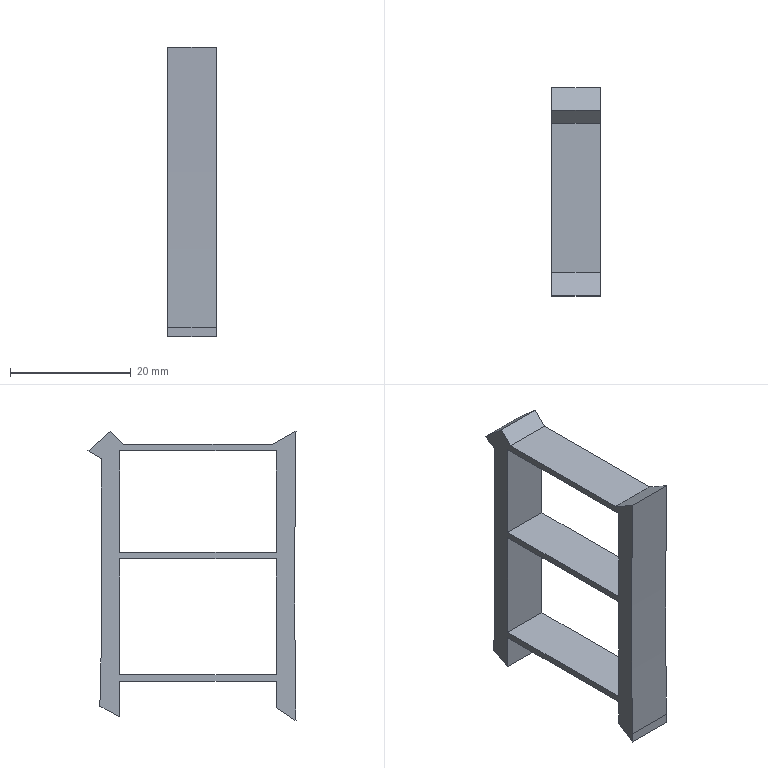Part | NX | features solid 2 | 1 solid | 23 faces | box 8 x 34.485 x 48.023 mm | volume 2991 mm3 | plane 21 | spline 2
STEP:
#1=CARTESIAN_POINT('',(2258.,545.559,-671.865));
#2=VERTEX_POINT('',#1);
#3=CARTESIAN_POINT('',(2258.,545.344,-630.831));
#4=VERTEX_POINT('',#3);
#5=CARTESIAN_POINT('',(2258.,545.559,-671.865));
#6=CARTESIAN_POINT('',(2258.,545.542,-671.425));
#7=CARTESIAN_POINT('',(2258.,545.525,-670.985));
#8=CARTESIAN_POINT('',(2258.,545.49,-670.091));
#9=CARTESIAN_POINT('',(2258.,545.48,-669.638));
#10=CARTESIAN_POINT('',(2258.,545.453,-668.717));
#11=CARTESIAN_POINT('',(2258.,545.44,-668.249));
#12=CARTESIAN_POINT('',(2258.,545.412,-667.308));
#13=CARTESIAN_POINT('',(2258.,545.405,-666.834));
#14=CARTESIAN_POINT('',(2258.,545.385,-665.872));
#15=CARTESIAN_POINT('',(2258.,545.382,-665.384));
#16=CARTESIAN_POINT('',(2258.,545.368,-664.395));
#17=CARTESIAN_POINT('',(2258.,545.361,-663.894));
#18=CARTESIAN_POINT('',(2258.,545.347,-662.884));
#19=CARTESIAN_POINT('',(2258.,545.347,-662.376));
#20=CARTESIAN_POINT('',(2258.,545.341,-661.346));
#21=CARTESIAN_POINT('',(2258.,545.344,-660.824));
#22=CARTESIAN_POINT('',(2258.,545.344,-650.478));
#23=CARTESIAN_POINT('',(2258.,545.344,-640.655));
#24=CARTESIAN_POINT('',(2258.,545.344,-630.831));
#25=B_SPLINE_CURVE_WITH_KNOTS('',3,(#5,#6,#7,#8,#9,#10,#11,#12,#13,#14,#15,#16,#17,#18,#19,#20,#21,#22,#23,#24),.UNSPECIFIED.,.F.,.F.,(4,2,2,2,2,2,2,2,2,4),(0.2635,0.2712,0.2791,0.2872,0.2954,0.3039,0.3126,0.3215,0.3305,0.5012),.UNSPECIFIED.);
#26=EDGE_CURVE('',#2,#4,#25,.T.);
#27=ORIENTED_EDGE('',*,*,#26,.F.);
#28=CARTESIAN_POINT('',(2250.,545.559,-671.865));
#29=VERTEX_POINT('',#28);
#30=CARTESIAN_POINT('',(2250.,545.559,-671.865));
#31=DIRECTION('',(1.,0.,0.));
#32=VECTOR('',#31,1000.);
#33=LINE('',#30,#32);
#34=EDGE_CURVE('',#29,#2,#33,.T.);
#35=ORIENTED_EDGE('',*,*,#34,.F.);
#36=CARTESIAN_POINT('',(2250.,545.344,-630.831));
#37=VERTEX_POINT('',#36);
#38=CARTESIAN_POINT('',(2250.,545.559,-671.865));
#39=CARTESIAN_POINT('',(2250.,545.542,-671.425));
#40=CARTESIAN_POINT('',(2250.,545.525,-670.985));
#41=CARTESIAN_POINT('',(2250.,545.49,-670.091));
#42=CARTESIAN_POINT('',(2250.,545.48,-669.638));
#43=CARTESIAN_POINT('',(2250.,545.453,-668.717));
#44=CARTESIAN_POINT('',(2250.,545.44,-668.249));
#45=CARTESIAN_POINT('',(2250.,545.412,-667.308));
#46=CARTESIAN_POINT('',(2250.,545.405,-666.834));
#47=CARTESIAN_POINT('',(2250.,545.385,-665.872));
#48=CARTESIAN_POINT('',(2250.,545.382,-665.384));
#49=CARTESIAN_POINT('',(2250.,545.368,-664.395));
#50=CARTESIAN_POINT('',(2250.,545.361,-663.894));
#51=CARTESIAN_POINT('',(2250.,545.347,-662.884));
#52=CARTESIAN_POINT('',(2250.,545.347,-662.376));
#53=CARTESIAN_POINT('',(2250.,545.341,-661.346));
#54=CARTESIAN_POINT('',(2250.,545.344,-660.824));
#55=CARTESIAN_POINT('',(2250.,545.344,-650.478));
#56=CARTESIAN_POINT('',(2250.,545.344,-640.655));
#57=CARTESIAN_POINT('',(2250.,545.344,-630.831));
#58=B_SPLINE_CURVE_WITH_KNOTS('',3,(#38,#39,#40,#41,#42,#43,#44,#45,#46,#47,#48,#49,#50,#51,#52,#53,#54,#55,#56,#57),.UNSPECIFIED.,.F.,.F.,(4,2,2,2,2,2,2,2,2,4),(0.2635,0.2712,0.2791,0.2872,0.2954,0.3039,0.3126,0.3215,0.3305,0.5012),.UNSPECIFIED.);
#59=EDGE_CURVE('',#29,#37,#58,.T.);
#60=ORIENTED_EDGE('',*,*,#59,.T.);
#61=CARTESIAN_POINT('',(2250.,545.344,-630.831));
#62=DIRECTION('',(1.,0.,0.));
#63=VECTOR('',#62,1000.);
#64=LINE('',#61,#63);
#65=EDGE_CURVE('',#37,#4,#64,.T.);
#66=ORIENTED_EDGE('',*,*,#65,.T.);
#67=EDGE_LOOP('',(#27,#35,#60,#66));
#68=FACE_BOUND('',#67,.T.);
#69=CARTESIAN_POINT('',(2250.,545.559,-671.865));
#70=CARTESIAN_POINT('',(2258.,545.559,-671.865));
#71=CARTESIAN_POINT('',(2250.,545.294,-665.031));
#72=CARTESIAN_POINT('',(2258.,545.294,-665.031));
#73=CARTESIAN_POINT('',(2250.,545.369,-651.348));
#74=CARTESIAN_POINT('',(2258.,545.369,-651.348));
#75=CARTESIAN_POINT('',(2250.,545.344,-637.671));
#76=CARTESIAN_POINT('',(2258.,545.344,-637.671));
#77=CARTESIAN_POINT('',(2250.,545.344,-630.831));
#78=CARTESIAN_POINT('',(2258.,545.344,-630.831));
#79=B_SPLINE_SURFACE_WITH_KNOTS('',3,1,((#69,#70),(#71,#72),(#73,#74),(#75,#76),(#77,#78)),.SURF_OF_LINEAR_EXTRUSION.,.F.,.F.,.F.,(4,1,4),(2,2),(0.2635,0.3824,0.5012),(0.,1.),.UNSPECIFIED.);
#80=ADVANCED_FACE('',(#68),#79,.T.);
#81=CARTESIAN_POINT('',(2258.,513.039,-626.247));
#82=VERTEX_POINT('',#81);
#83=CARTESIAN_POINT('',(2258.,513.07,-672.643));
#84=VERTEX_POINT('',#83);
#85=CARTESIAN_POINT('',(2258.,513.039,-626.247));
#86=CARTESIAN_POINT('',(2258.,513.049,-626.8));
#87=CARTESIAN_POINT('',(2258.,513.06,-627.352));
#88=CARTESIAN_POINT('',(2258.,513.08,-628.447));
#89=CARTESIAN_POINT('',(2258.,513.083,-628.99));
#90=CARTESIAN_POINT('',(2258.,513.097,-630.071));
#91=CARTESIAN_POINT('',(2258.,513.104,-630.61));
#92=CARTESIAN_POINT('',(2258.,513.117,-631.681));
#93=CARTESIAN_POINT('',(2258.,513.124,-632.213));
#94=CARTESIAN_POINT('',(2258.,513.138,-633.27));
#95=CARTESIAN_POINT('',(2258.,513.145,-633.796));
#96=CARTESIAN_POINT('',(2258.,513.158,-634.839));
#97=CARTESIAN_POINT('',(2258.,513.165,-635.358));
#98=CARTESIAN_POINT('',(2258.,513.179,-636.391));
#99=CARTESIAN_POINT('',(2258.,513.186,-636.906));
#100=CARTESIAN_POINT('',(2258.,513.199,-637.926));
#101=CARTESIAN_POINT('',(2258.,513.199,-638.431));
#102=CARTESIAN_POINT('',(2258.,513.206,-639.434));
#103=CARTESIAN_POINT('',(2258.,513.21,-639.932));
#104=CARTESIAN_POINT('',(2258.,513.216,-640.924));
#105=CARTESIAN_POINT('',(2258.,513.22,-641.419));
#106=CARTESIAN_POINT('',(2258.,513.227,-642.398));
#107=CARTESIAN_POINT('',(2258.,513.23,-642.882));
#108=CARTESIAN_POINT('',(2258.,513.237,-643.848));
#109=CARTESIAN_POINT('',(2258.,513.24,-644.328));
#110=CARTESIAN_POINT('',(2258.,513.247,-645.284));
#111=CARTESIAN_POINT('',(2258.,513.251,-645.758));
#112=CARTESIAN_POINT('',(2258.,513.257,-646.696));
#113=CARTESIAN_POINT('',(2258.,513.254,-647.16));
#114=CARTESIAN_POINT('',(2258.,513.254,-648.084));
#115=CARTESIAN_POINT('',(2258.,513.254,-648.544));
#116=CARTESIAN_POINT('',(2258.,513.254,-649.459));
#117=CARTESIAN_POINT('',(2258.,513.254,-649.912));
#118=CARTESIAN_POINT('',(2258.,513.254,-650.819));
#119=CARTESIAN_POINT('',(2258.,513.254,-651.273));
#120=CARTESIAN_POINT('',(2258.,513.254,-652.187));
#121=CARTESIAN_POINT('',(2258.,513.254,-652.648));
#122=CARTESIAN_POINT('',(2258.,513.254,-653.572));
#123=CARTESIAN_POINT('',(2258.,513.254,-654.036));
#124=CARTESIAN_POINT('',(2258.,513.254,-654.971));
#125=CARTESIAN_POINT('',(2258.,513.247,-655.441));
#126=CARTESIAN_POINT('',(2258.,513.24,-656.39));
#127=CARTESIAN_POINT('',(2258.,513.237,-656.867));
#128=CARTESIAN_POINT('',(2258.,513.23,-657.829));
#129=CARTESIAN_POINT('',(2258.,513.227,-658.313));
#130=CARTESIAN_POINT('',(2258.,513.22,-659.285));
#131=CARTESIAN_POINT('',(2258.,513.216,-659.773));
#132=CARTESIAN_POINT('',(2258.,513.21,-660.756));
#133=CARTESIAN_POINT('',(2258.,513.206,-661.25));
#134=CARTESIAN_POINT('',(2258.,513.199,-662.246));
#135=CARTESIAN_POINT('',(2258.,513.196,-662.748));
#136=CARTESIAN_POINT('',(2258.,513.189,-663.757));
#137=CARTESIAN_POINT('',(2258.,513.179,-664.265));
#138=CARTESIAN_POINT('',(2258.,513.165,-665.285));
#139=CARTESIAN_POINT('',(2258.,513.158,-665.797));
#140=CARTESIAN_POINT('',(2258.,513.145,-666.827));
#141=CARTESIAN_POINT('',(2258.,513.138,-667.345));
#142=CARTESIAN_POINT('',(2258.,513.124,-668.389));
#143=CARTESIAN_POINT('',(2258.,513.118,-668.914));
#144=CARTESIAN_POINT('',(2258.,513.104,-669.972));
#145=CARTESIAN_POINT('',(2258.,513.097,-670.504));
#146=CARTESIAN_POINT('',(2258.,513.083,-671.572));
#147=CARTESIAN_POINT('',(2258.,513.077,-672.107));
#148=CARTESIAN_POINT('',(2258.,513.07,-672.643));
#149=B_SPLINE_CURVE_WITH_KNOTS('',3,(#85,#86,#87,#88,#89,#90,#91,#92,#93,#94,#95,#96,#97,#98,#99,#100,#101,#102,#103,#104,#105,#106,#107,#108,#109,#110,#111,#112,#113,#114,#115,#116,#117,#118,#119,#120,#121,#122,#123,#124,#125,#126,#127,#128,#129,#130,#131,#132,#133,#134,#135,#136,#137,#138,#139,#140,#141,#142,#143,#144,#145,#146,#147,#148),.UNSPECIFIED.,.F.,.F.,(4,2,2,2,2,2,2,2,2,2,2,2,2,2,2,2,2,2,2,2,2,2,2,2,2,2,2,2,2,2,2,4),(0.7313,0.7409,0.7503,0.7597,0.7689,0.7781,0.7871,0.796,0.8048,0.8134,0.822,0.8304,0.8388,0.847,0.8551,0.8631,0.871,0.8789,0.8869,0.8949,0.9031,0.9114,0.9198,0.9283,0.9369,0.9456,0.9544,0.9633,0.9723,0.9814,0.9907,1.),.UNSPECIFIED.);
#150=EDGE_CURVE('',#82,#84,#149,.T.);
#151=ORIENTED_EDGE('',*,*,#150,.F.);
#152=CARTESIAN_POINT('',(2250.,513.039,-626.247));
#153=VERTEX_POINT('',#152);
#154=CARTESIAN_POINT('',(2250.,513.039,-626.247));
#155=DIRECTION('',(1.,0.,0.));
#156=VECTOR('',#155,1000.);
#157=LINE('',#154,#156);
#158=EDGE_CURVE('',#153,#82,#157,.T.);
#159=ORIENTED_EDGE('',*,*,#158,.F.);
#160=CARTESIAN_POINT('',(2250.,513.07,-672.643));
#161=VERTEX_POINT('',#160);
#162=CARTESIAN_POINT('',(2250.,513.039,-626.247));
#163=CARTESIAN_POINT('',(2250.,513.049,-626.8));
#164=CARTESIAN_POINT('',(2250.,513.06,-627.352));
#165=CARTESIAN_POINT('',(2250.,513.08,-628.447));
#166=CARTESIAN_POINT('',(2250.,513.083,-628.99));
#167=CARTESIAN_POINT('',(2250.,513.097,-630.071));
#168=CARTESIAN_POINT('',(2250.,513.104,-630.61));
#169=CARTESIAN_POINT('',(2250.,513.117,-631.681));
#170=CARTESIAN_POINT('',(2250.,513.124,-632.213));
#171=CARTESIAN_POINT('',(2250.,513.138,-633.27));
#172=CARTESIAN_POINT('',(2250.,513.145,-633.796));
#173=CARTESIAN_POINT('',(2250.,513.158,-634.839));
#174=CARTESIAN_POINT('',(2250.,513.165,-635.358));
#175=CARTESIAN_POINT('',(2250.,513.179,-636.391));
#176=CARTESIAN_POINT('',(2250.,513.186,-636.906));
#177=CARTESIAN_POINT('',(2250.,513.199,-637.926));
#178=CARTESIAN_POINT('',(2250.,513.199,-638.431));
#179=CARTESIAN_POINT('',(2250.,513.206,-639.434));
#180=CARTESIAN_POINT('',(2250.,513.21,-639.932));
#181=CARTESIAN_POINT('',(2250.,513.216,-640.924));
#182=CARTESIAN_POINT('',(2250.,513.22,-641.419));
#183=CARTESIAN_POINT('',(2250.,513.227,-642.398));
#184=CARTESIAN_POINT('',(2250.,513.23,-642.882));
#185=CARTESIAN_POINT('',(2250.,513.237,-643.848));
#186=CARTESIAN_POINT('',(2250.,513.24,-644.328));
#187=CARTESIAN_POINT('',(2250.,513.247,-645.284));
#188=CARTESIAN_POINT('',(2250.,513.251,-645.758));
#189=CARTESIAN_POINT('',(2250.,513.257,-646.696));
#190=CARTESIAN_POINT('',(2250.,513.254,-647.16));
#191=CARTESIAN_POINT('',(2250.,513.254,-648.084));
#192=CARTESIAN_POINT('',(2250.,513.254,-648.544));
#193=CARTESIAN_POINT('',(2250.,513.254,-649.459));
#194=CARTESIAN_POINT('',(2250.,513.254,-649.912));
#195=CARTESIAN_POINT('',(2250.,513.254,-650.819));
#196=CARTESIAN_POINT('',(2250.,513.254,-651.273));
#197=CARTESIAN_POINT('',(2250.,513.254,-652.187));
#198=CARTESIAN_POINT('',(2250.,513.254,-652.648));
#199=CARTESIAN_POINT('',(2250.,513.254,-653.572));
#200=CARTESIAN_POINT('',(2250.,513.254,-654.036));
#201=CARTESIAN_POINT('',(2250.,513.254,-654.971));
#202=CARTESIAN_POINT('',(2250.,513.247,-655.441));
#203=CARTESIAN_POINT('',(2250.,513.24,-656.39));
#204=CARTESIAN_POINT('',(2250.,513.237,-656.867));
#205=CARTESIAN_POINT('',(2250.,513.23,-657.829));
#206=CARTESIAN_POINT('',(2250.,513.227,-658.313));
#207=CARTESIAN_POINT('',(2250.,513.22,-659.285));
#208=CARTESIAN_POINT('',(2250.,513.216,-659.773));
#209=CARTESIAN_POINT('',(2250.,513.21,-660.756));
#210=CARTESIAN_POINT('',(2250.,513.206,-661.25));
#211=CARTESIAN_POINT('',(2250.,513.199,-662.246));
#212=CARTESIAN_POINT('',(2250.,513.196,-662.748));
#213=CARTESIAN_POINT('',(2250.,513.189,-663.757));
#214=CARTESIAN_POINT('',(2250.,513.179,-664.265));
#215=CARTESIAN_POINT('',(2250.,513.165,-665.285));
#216=CARTESIAN_POINT('',(2250.,513.158,-665.797));
#217=CARTESIAN_POINT('',(2250.,513.145,-666.827));
#218=CARTESIAN_POINT('',(2250.,513.138,-667.345));
#219=CARTESIAN_POINT('',(2250.,513.124,-668.389));
#220=CARTESIAN_POINT('',(2250.,513.118,-668.914));
#221=CARTESIAN_POINT('',(2250.,513.104,-669.972));
#222=CARTESIAN_POINT('',(2250.,513.097,-670.504));
#223=CARTESIAN_POINT('',(2250.,513.083,-671.572));
#224=CARTESIAN_POINT('',(2250.,513.077,-672.107));
#225=CARTESIAN_POINT('',(2250.,513.07,-672.643));
#226=B_SPLINE_CURVE_WITH_KNOTS('',3,(#162,#163,#164,#165,#166,#167,#168,#169,#170,#171,#172,#173,#174,#175,#176,#177,#178,#179,#180,#181,#182,#183,#184,#185,#186,#187,#188,#189,#190,#191,#192,#193,#194,#195,#196,#197,#198,#199,#200,#201,#202,#203,#204,#205,#206,#207,#208,#209,#210,#211,#212,#213,#214,#215,#216,#217,#218,#219,#220,#221,#222,#223,#224,#225),.UNSPECIFIED.,.F.,.F.,(4,2,2,2,2,2,2,2,2,2,2,2,2,2,2,2,2,2,2,2,2,2,2,2,2,2,2,2,2,2,2,4),(0.7313,0.7409,0.7503,0.7597,0.7689,0.7781,0.7871,0.796,0.8048,0.8134,0.822,0.8304,0.8388,0.847,0.8551,0.8631,0.871,0.8789,0.8869,0.8949,0.9031,0.9114,0.9198,0.9283,0.9369,0.9456,0.9544,0.9633,0.9723,0.9814,0.9907,1.),.UNSPECIFIED.);
#227=EDGE_CURVE('',#153,#161,#226,.T.);
#228=ORIENTED_EDGE('',*,*,#227,.T.);
#229=CARTESIAN_POINT('',(2250.,513.07,-672.643));
#230=DIRECTION('',(1.,0.,0.));
#231=VECTOR('',#230,1000.);
#232=LINE('',#229,#231);
#233=EDGE_CURVE('',#161,#84,#232,.T.);
#234=ORIENTED_EDGE('',*,*,#233,.T.);
#235=EDGE_LOOP('',(#151,#159,#228,#234));
#236=FACE_BOUND('',#235,.T.);
#237=CARTESIAN_POINT('',(2250.,513.039,-626.247));
#238=CARTESIAN_POINT('',(2258.,513.039,-626.247));
#239=CARTESIAN_POINT('',(2250.,513.182,-633.979));
#240=CARTESIAN_POINT('',(2258.,513.182,-633.979));
#241=CARTESIAN_POINT('',(2250.,513.333,-649.445));
#242=CARTESIAN_POINT('',(2258.,513.333,-649.445));
#243=CARTESIAN_POINT('',(2250.,513.168,-664.91));
#244=CARTESIAN_POINT('',(2258.,513.168,-664.91));
#245=CARTESIAN_POINT('',(2250.,513.07,-672.643));
#246=CARTESIAN_POINT('',(2258.,513.07,-672.643));
#247=B_SPLINE_SURFACE_WITH_KNOTS('',3,1,((#237,#238),(#239,#240),(#241,#242),(#243,#244),(#245,#246)),.SURF_OF_LINEAR_EXTRUSION.,.F.,.F.,.F.,(4,1,4),(2,2),(0.7313,0.8656,1.),(0.,1.),.UNSPECIFIED.);
#248=ADVANCED_FACE('',(#236),#247,.T.);
#249=CARTESIAN_POINT('',(2250.,516.314,-629.522));
#250=VERTEX_POINT('',#249);
#251=CARTESIAN_POINT('',(2258.,516.314,-629.522));
#252=VERTEX_POINT('',#251);
#253=CARTESIAN_POINT('',(2250.,516.314,-629.522));
#254=DIRECTION('',(1.,0.,0.));
#255=VECTOR('',#254,1000.);
#256=LINE('',#253,#255);
#257=EDGE_CURVE('',#250,#252,#256,.T.);
#258=ORIENTED_EDGE('',*,*,#257,.T.);
#259=CARTESIAN_POINT('',(2258.,516.314,-646.334));
#260=VERTEX_POINT('',#259);
#261=CARTESIAN_POINT('',(2258.,516.314,-646.334));
#262=DIRECTION('',(0.,0.,-1.));
#263=VECTOR('',#262,1000.);
#264=LINE('',#261,#263);
#265=EDGE_CURVE('',#252,#260,#264,.T.);
#266=ORIENTED_EDGE('',*,*,#265,.T.);
#267=CARTESIAN_POINT('',(2250.,516.314,-646.334));
#268=VERTEX_POINT('',#267);
#269=CARTESIAN_POINT('',(2250.,516.314,-646.334));
#270=DIRECTION('',(1.,0.,0.));
#271=VECTOR('',#270,1000.);
#272=LINE('',#269,#271);
#273=EDGE_CURVE('',#268,#260,#272,.T.);
#274=ORIENTED_EDGE('',*,*,#273,.F.);
#275=CARTESIAN_POINT('',(2250.,516.314,-646.334));
#276=CARTESIAN_POINT('',(2250.,516.314,-640.73));
#277=CARTESIAN_POINT('',(2250.,516.314,-635.126));
#278=CARTESIAN_POINT('',(2250.,516.314,-629.522));
#279=B_SPLINE_CURVE_WITH_KNOTS('',3,(#275,#276,#277,#278),.UNSPECIFIED.,.F.,.F.,(4,4),(0.,0.1965),.PIECEWISE_BEZIER_KNOTS.);
#280=EDGE_CURVE('',#268,#250,#279,.T.);
#281=ORIENTED_EDGE('',*,*,#280,.T.);
#282=EDGE_LOOP('',(#258,#266,#274,#281));
#283=FACE_BOUND('',#282,.T.);
#284=CARTESIAN_POINT('',(2250.,516.314,-646.334));
#285=DIRECTION('',(0.,-1.,0.));
#286=DIRECTION('',(-1.,0.,0.));
#287=AXIS2_PLACEMENT_3D('',#284,#285,#286);
#288=PLANE('',#287);
#289=ADVANCED_FACE('',(#283),#288,.F.);
#290=CARTESIAN_POINT('',(2250.,542.284,-629.522));
#291=VERTEX_POINT('',#290);
#292=CARTESIAN_POINT('',(2258.,542.284,-629.522));
#293=VERTEX_POINT('',#292);
#294=CARTESIAN_POINT('',(2250.,542.284,-629.522));
#295=DIRECTION('',(1.,0.,0.));
#296=VECTOR('',#295,1000.);
#297=LINE('',#294,#296);
#298=EDGE_CURVE('',#291,#293,#297,.T.);
#299=ORIENTED_EDGE('',*,*,#298,.T.);
#300=CARTESIAN_POINT('',(2258.,516.314,-629.522));
#301=DIRECTION('',(0.,-1.,0.));
#302=VECTOR('',#301,1000.);
#303=LINE('',#300,#302);
#304=EDGE_CURVE('',#293,#252,#303,.T.);
#305=ORIENTED_EDGE('',*,*,#304,.T.);
#306=ORIENTED_EDGE('',*,*,#257,.F.);
#307=CARTESIAN_POINT('',(2250.,516.314,-629.522));
#308=CARTESIAN_POINT('',(2250.,524.971,-629.522));
#309=CARTESIAN_POINT('',(2250.,533.627,-629.522));
#310=CARTESIAN_POINT('',(2250.,542.284,-629.522));
#311=B_SPLINE_CURVE_WITH_KNOTS('',3,(#307,#308,#309,#310),.UNSPECIFIED.,.F.,.F.,(4,4),(0.1965,0.5),.PIECEWISE_BEZIER_KNOTS.);
#312=EDGE_CURVE('',#250,#291,#311,.T.);
#313=ORIENTED_EDGE('',*,*,#312,.T.);
#314=EDGE_LOOP('',(#299,#305,#306,#313));
#315=FACE_BOUND('',#314,.T.);
#316=CARTESIAN_POINT('',(2250.,516.314,-629.522));
#317=DIRECTION('',(0.,0.,1.));
#318=DIRECTION('',(-1.,0.,0.));
#319=AXIS2_PLACEMENT_3D('',#316,#317,#318);
#320=PLANE('',#319);
#321=ADVANCED_FACE('',(#315),#320,.F.);
#322=CARTESIAN_POINT('',(2250.,542.284,-646.334));
#323=VERTEX_POINT('',#322);
#324=CARTESIAN_POINT('',(2258.,542.284,-646.334));
#325=VERTEX_POINT('',#324);
#326=CARTESIAN_POINT('',(2250.,542.284,-646.334));
#327=DIRECTION('',(1.,0.,0.));
#328=VECTOR('',#327,1000.);
#329=LINE('',#326,#328);
#330=EDGE_CURVE('',#323,#325,#329,.T.);
#331=ORIENTED_EDGE('',*,*,#330,.T.);
#332=CARTESIAN_POINT('',(2258.,542.284,-629.522));
#333=DIRECTION('',(0.,0.,1.));
#334=VECTOR('',#333,1000.);
#335=LINE('',#332,#334);
#336=EDGE_CURVE('',#325,#293,#335,.T.);
#337=ORIENTED_EDGE('',*,*,#336,.T.);
#338=ORIENTED_EDGE('',*,*,#298,.F.);
#339=CARTESIAN_POINT('',(2250.,542.284,-629.522));
#340=CARTESIAN_POINT('',(2250.,542.284,-635.126));
#341=CARTESIAN_POINT('',(2250.,542.284,-640.73));
#342=CARTESIAN_POINT('',(2250.,542.284,-646.334));
#343=B_SPLINE_CURVE_WITH_KNOTS('',3,(#339,#340,#341,#342),.UNSPECIFIED.,.F.,.F.,(4,4),(0.5,0.6965),.PIECEWISE_BEZIER_KNOTS.);
#344=EDGE_CURVE('',#291,#323,#343,.T.);
#345=ORIENTED_EDGE('',*,*,#344,.T.);
#346=EDGE_LOOP('',(#331,#337,#338,#345));
#347=FACE_BOUND('',#346,.T.);
#348=CARTESIAN_POINT('',(2250.,542.284,-629.522));
#349=DIRECTION('',(0.,1.,0.));
#350=DIRECTION('',(1.,0.,0.));
#351=AXIS2_PLACEMENT_3D('',#348,#349,#350);
#352=PLANE('',#351);
#353=ADVANCED_FACE('',(#347),#352,.F.);
#354=CARTESIAN_POINT('',(2250.,516.314,-647.419));
#355=VERTEX_POINT('',#354);
#356=CARTESIAN_POINT('',(2258.,516.314,-647.419));
#357=VERTEX_POINT('',#356);
#358=CARTESIAN_POINT('',(2250.,516.314,-647.419));
#359=DIRECTION('',(1.,0.,0.));
#360=VECTOR('',#359,1000.);
#361=LINE('',#358,#360);
#362=EDGE_CURVE('',#355,#357,#361,.T.);
#363=ORIENTED_EDGE('',*,*,#362,.T.);
#364=CARTESIAN_POINT('',(2258.,516.314,-666.626));
#365=VERTEX_POINT('',#364);
#366=CARTESIAN_POINT('',(2258.,516.314,-666.626));
#367=DIRECTION('',(0.,0.,-1.));
#368=VECTOR('',#367,1000.);
#369=LINE('',#366,#368);
#370=EDGE_CURVE('',#357,#365,#369,.T.);
#371=ORIENTED_EDGE('',*,*,#370,.T.);
#372=CARTESIAN_POINT('',(2250.,516.314,-666.626));
#373=VERTEX_POINT('',#372);
#374=CARTESIAN_POINT('',(2250.,516.314,-666.626));
#375=DIRECTION('',(1.,0.,0.));
#376=VECTOR('',#375,1000.);
#377=LINE('',#374,#376);
#378=EDGE_CURVE('',#373,#365,#377,.T.);
#379=ORIENTED_EDGE('',*,*,#378,.F.);
#380=CARTESIAN_POINT('',(2250.,516.314,-666.626));
#381=CARTESIAN_POINT('',(2250.,516.314,-660.223));
#382=CARTESIAN_POINT('',(2250.,516.314,-653.821));
#383=CARTESIAN_POINT('',(2250.,516.314,-647.419));
#384=B_SPLINE_CURVE_WITH_KNOTS('',3,(#380,#381,#382,#383),.UNSPECIFIED.,.F.,.F.,(4,4),(0.,0.2126),.PIECEWISE_BEZIER_KNOTS.);
#385=EDGE_CURVE('',#373,#355,#384,.T.);
#386=ORIENTED_EDGE('',*,*,#385,.T.);
#387=EDGE_LOOP('',(#363,#371,#379,#386));
#388=FACE_BOUND('',#387,.T.);
#389=CARTESIAN_POINT('',(2250.,516.314,-666.626));
#390=DIRECTION('',(0.,-1.,0.));
#391=DIRECTION('',(-1.,0.,0.));
#392=AXIS2_PLACEMENT_3D('',#389,#390,#391);
#393=PLANE('',#392);
#394=ADVANCED_FACE('',(#388),#393,.F.);
#395=CARTESIAN_POINT('',(2250.,542.284,-647.419));
#396=VERTEX_POINT('',#395);
#397=CARTESIAN_POINT('',(2258.,542.284,-647.419));
#398=VERTEX_POINT('',#397);
#399=CARTESIAN_POINT('',(2250.,542.284,-647.419));
#400=DIRECTION('',(1.,0.,0.));
#401=VECTOR('',#400,1000.);
#402=LINE('',#399,#401);
#403=EDGE_CURVE('',#396,#398,#402,.T.);
#404=ORIENTED_EDGE('',*,*,#403,.T.);
#405=CARTESIAN_POINT('',(2258.,516.314,-647.419));
#406=DIRECTION('',(0.,-1.,0.));
#407=VECTOR('',#406,1000.);
#408=LINE('',#405,#407);
#409=EDGE_CURVE('',#398,#357,#408,.T.);
#410=ORIENTED_EDGE('',*,*,#409,.T.);
#411=ORIENTED_EDGE('',*,*,#362,.F.);
#412=CARTESIAN_POINT('',(2250.,516.314,-647.419));
#413=CARTESIAN_POINT('',(2250.,524.971,-647.419));
#414=CARTESIAN_POINT('',(2250.,533.627,-647.419));
#415=CARTESIAN_POINT('',(2250.,542.284,-647.419));
#416=B_SPLINE_CURVE_WITH_KNOTS('',3,(#412,#413,#414,#415),.UNSPECIFIED.,.F.,.F.,(4,4),(0.2126,0.5),.PIECEWISE_BEZIER_KNOTS.);
#417=EDGE_CURVE('',#355,#396,#416,.T.);
#418=ORIENTED_EDGE('',*,*,#417,.T.);
#419=EDGE_LOOP('',(#404,#410,#411,#418));
#420=FACE_BOUND('',#419,.T.);
#421=CARTESIAN_POINT('',(2250.,516.314,-647.419));
#422=DIRECTION('',(0.,0.,1.));
#423=DIRECTION('',(-1.,0.,0.));
#424=AXIS2_PLACEMENT_3D('',#421,#422,#423);
#425=PLANE('',#424);
#426=ADVANCED_FACE('',(#420),#425,.F.);
#427=CARTESIAN_POINT('',(2250.,542.284,-666.626));
#428=VERTEX_POINT('',#427);
#429=CARTESIAN_POINT('',(2258.,542.284,-666.626));
#430=VERTEX_POINT('',#429);
#431=CARTESIAN_POINT('',(2250.,542.284,-666.626));
#432=DIRECTION('',(1.,0.,0.));
#433=VECTOR('',#432,1000.);
#434=LINE('',#431,#433);
#435=EDGE_CURVE('',#428,#430,#434,.T.);
#436=ORIENTED_EDGE('',*,*,#435,.T.);
#437=CARTESIAN_POINT('',(2258.,542.284,-647.419));
#438=DIRECTION('',(0.,0.,1.));
#439=VECTOR('',#438,1000.);
#440=LINE('',#437,#439);
#441=EDGE_CURVE('',#430,#398,#440,.T.);
#442=ORIENTED_EDGE('',*,*,#441,.T.);
#443=ORIENTED_EDGE('',*,*,#403,.F.);
#444=CARTESIAN_POINT('',(2250.,542.284,-647.419));
#445=CARTESIAN_POINT('',(2250.,542.284,-653.821));
#446=CARTESIAN_POINT('',(2250.,542.284,-660.223));
#447=CARTESIAN_POINT('',(2250.,542.284,-666.626));
#448=B_SPLINE_CURVE_WITH_KNOTS('',3,(#444,#445,#446,#447),.UNSPECIFIED.,.F.,.F.,(4,4),(0.5,0.7126),.PIECEWISE_BEZIER_KNOTS.);
#449=EDGE_CURVE('',#396,#428,#448,.T.);
#450=ORIENTED_EDGE('',*,*,#449,.T.);
#451=EDGE_LOOP('',(#436,#442,#443,#450));
#452=FACE_BOUND('',#451,.T.);
#453=CARTESIAN_POINT('',(2250.,542.284,-647.419));
#454=DIRECTION('',(0.,1.,0.));
#455=DIRECTION('',(1.,0.,0.));
#456=AXIS2_PLACEMENT_3D('',#453,#454,#455);
#457=PLANE('',#456);
#458=ADVANCED_FACE('',(#452),#457,.F.);
#459=CARTESIAN_POINT('',(2250.,513.039,-674.27));
#460=VERTEX_POINT('',#459);
#461=CARTESIAN_POINT('',(2258.,513.039,-674.27));
#462=VERTEX_POINT('',#461);
#463=CARTESIAN_POINT('',(2250.,513.039,-674.27));
#464=DIRECTION('',(1.,0.,0.));
#465=VECTOR('',#464,1000.);
#466=LINE('',#463,#465);
#467=EDGE_CURVE('',#460,#462,#466,.T.);
#468=ORIENTED_EDGE('',*,*,#467,.T.);
#469=CARTESIAN_POINT('',(2258.,513.07,-672.643));
#470=DIRECTION('',(0.,0.01886,0.9998));
#471=VECTOR('',#470,1000.);
#472=LINE('',#469,#471);
#473=EDGE_CURVE('',#462,#84,#472,.T.);
#474=ORIENTED_EDGE('',*,*,#473,.T.);
#475=ORIENTED_EDGE('',*,*,#233,.F.);
#476=CARTESIAN_POINT('',(2250.,513.07,-672.643));
#477=CARTESIAN_POINT('',(2250.,513.06,-673.185));
#478=CARTESIAN_POINT('',(2250.,513.049,-673.727));
#479=CARTESIAN_POINT('',(2250.,513.039,-674.27));
#480=B_SPLINE_CURVE_WITH_KNOTS('',3,(#476,#477,#478,#479),.UNSPECIFIED.,.F.,.F.,(4,4),(0.,0.009424),.PIECEWISE_BEZIER_KNOTS.);
#481=EDGE_CURVE('',#161,#460,#480,.T.);
#482=ORIENTED_EDGE('',*,*,#481,.T.);
#483=EDGE_LOOP('',(#468,#474,#475,#482));
#484=FACE_BOUND('',#483,.T.);
#485=CARTESIAN_POINT('',(2250.,513.07,-672.643));
#486=DIRECTION('',(0.,0.9998,-0.01886));
#487=DIRECTION('',(0.,0.01886,0.9998));
#488=AXIS2_PLACEMENT_3D('',#485,#486,#487);
#489=PLANE('',#488);
#490=ADVANCED_FACE('',(#484),#489,.F.);
#491=CARTESIAN_POINT('',(2250.,516.314,-672.09));
#492=VERTEX_POINT('',#491);
#493=CARTESIAN_POINT('',(2258.,516.314,-672.09));
#494=VERTEX_POINT('',#493);
#495=CARTESIAN_POINT('',(2250.,516.314,-672.09));
#496=DIRECTION('',(1.,0.,0.));
#497=VECTOR('',#496,1000.);
#498=LINE('',#495,#497);
#499=EDGE_CURVE('',#492,#494,#498,.T.);
#500=ORIENTED_EDGE('',*,*,#499,.T.);
#501=CARTESIAN_POINT('',(2258.,513.039,-674.27));
#502=DIRECTION('',(0.,-0.8325,-0.5541));
#503=VECTOR('',#502,1000.);
#504=LINE('',#501,#503);
#505=EDGE_CURVE('',#494,#462,#504,.T.);
#506=ORIENTED_EDGE('',*,*,#505,.T.);
#507=ORIENTED_EDGE('',*,*,#467,.F.);
#508=CARTESIAN_POINT('',(2250.,513.039,-674.27));
#509=CARTESIAN_POINT('',(2250.,514.131,-673.543));
#510=CARTESIAN_POINT('',(2250.,515.222,-672.817));
#511=CARTESIAN_POINT('',(2250.,516.314,-672.09));
#512=B_SPLINE_CURVE_WITH_KNOTS('',3,(#508,#509,#510,#511),.UNSPECIFIED.,.F.,.F.,(4,4),(0.009424,0.0322),.PIECEWISE_BEZIER_KNOTS.);
#513=EDGE_CURVE('',#460,#492,#512,.T.);
#514=ORIENTED_EDGE('',*,*,#513,.T.);
#515=EDGE_LOOP('',(#500,#506,#507,#514));
#516=FACE_BOUND('',#515,.T.);
#517=CARTESIAN_POINT('',(2250.,513.039,-674.27));
#518=DIRECTION('',(0.,-0.5541,0.8325));
#519=DIRECTION('',(0.,-0.8325,-0.5541));
#520=AXIS2_PLACEMENT_3D('',#517,#518,#519);
#521=PLANE('',#520);
#522=ADVANCED_FACE('',(#516),#521,.F.);
#523=CARTESIAN_POINT('',(2250.,516.314,-667.721));
#524=VERTEX_POINT('',#523);
#525=CARTESIAN_POINT('',(2258.,516.314,-667.721));
#526=VERTEX_POINT('',#525);
#527=CARTESIAN_POINT('',(2250.,516.314,-667.721));
#528=DIRECTION('',(1.,0.,0.));
#529=VECTOR('',#528,1000.);
#530=LINE('',#527,#529);
#531=EDGE_CURVE('',#524,#526,#530,.T.);
#532=ORIENTED_EDGE('',*,*,#531,.T.);
#533=CARTESIAN_POINT('',(2258.,516.314,-672.09));
#534=DIRECTION('',(0.,0.,-1.));
#535=VECTOR('',#534,1000.);
#536=LINE('',#533,#535);
#537=EDGE_CURVE('',#526,#494,#536,.T.);
#538=ORIENTED_EDGE('',*,*,#537,.T.);
#539=ORIENTED_EDGE('',*,*,#499,.F.);
#540=CARTESIAN_POINT('',(2250.,516.314,-672.09));
#541=CARTESIAN_POINT('',(2250.,516.314,-670.634));
#542=CARTESIAN_POINT('',(2250.,516.314,-669.177));
#543=CARTESIAN_POINT('',(2250.,516.314,-667.721));
#544=B_SPLINE_CURVE_WITH_KNOTS('',3,(#540,#541,#542,#543),.UNSPECIFIED.,.F.,.F.,(4,4),(0.0322,0.05751),.PIECEWISE_BEZIER_KNOTS.);
#545=EDGE_CURVE('',#492,#524,#544,.T.);
#546=ORIENTED_EDGE('',*,*,#545,.T.);
#547=EDGE_LOOP('',(#532,#538,#539,#546));
#548=FACE_BOUND('',#547,.T.);
#549=CARTESIAN_POINT('',(2250.,516.314,-672.09));
#550=DIRECTION('',(0.,-1.,0.));
#551=DIRECTION('',(-1.,0.,0.));
#552=AXIS2_PLACEMENT_3D('',#549,#550,#551);
#553=PLANE('',#552);
#554=ADVANCED_FACE('',(#548),#553,.F.);
#555=CARTESIAN_POINT('',(2250.,542.284,-667.721));
#556=VERTEX_POINT('',#555);
#557=CARTESIAN_POINT('',(2258.,542.284,-667.721));
#558=VERTEX_POINT('',#557);
#559=CARTESIAN_POINT('',(2250.,542.284,-667.721));
#560=DIRECTION('',(1.,0.,0.));
#561=VECTOR('',#560,1000.);
#562=LINE('',#559,#561);
#563=EDGE_CURVE('',#556,#558,#562,.T.);
#564=ORIENTED_EDGE('',*,*,#563,.T.);
#565=CARTESIAN_POINT('',(2258.,516.314,-667.721));
#566=DIRECTION('',(0.,-1.,0.));
#567=VECTOR('',#566,1000.);
#568=LINE('',#565,#567);
#569=EDGE_CURVE('',#558,#526,#568,.T.);
#570=ORIENTED_EDGE('',*,*,#569,.T.);
#571=ORIENTED_EDGE('',*,*,#531,.F.);
#572=CARTESIAN_POINT('',(2250.,516.314,-667.721));
#573=CARTESIAN_POINT('',(2250.,524.971,-667.721));
#574=CARTESIAN_POINT('',(2250.,533.627,-667.721));
#575=CARTESIAN_POINT('',(2250.,542.284,-667.721));
#576=B_SPLINE_CURVE_WITH_KNOTS('',3,(#572,#573,#574,#575),.UNSPECIFIED.,.F.,.F.,(4,4),(0.05751,0.2079),.PIECEWISE_BEZIER_KNOTS.);
#577=EDGE_CURVE('',#524,#556,#576,.T.);
#578=ORIENTED_EDGE('',*,*,#577,.T.);
#579=EDGE_LOOP('',(#564,#570,#571,#578));
#580=FACE_BOUND('',#579,.T.);
#581=CARTESIAN_POINT('',(2250.,516.314,-667.721));
#582=DIRECTION('',(0.,0.,1.));
#583=DIRECTION('',(-1.,0.,0.));
#584=AXIS2_PLACEMENT_3D('',#581,#582,#583);
#585=PLANE('',#584);
#586=ADVANCED_FACE('',(#580),#585,.F.);
#587=CARTESIAN_POINT('',(2250.,542.284,-673.615));
#588=VERTEX_POINT('',#587);
#589=CARTESIAN_POINT('',(2258.,542.284,-673.615));
#590=VERTEX_POINT('',#589);
#591=CARTESIAN_POINT('',(2250.,542.284,-673.615));
#592=DIRECTION('',(1.,0.,0.));
#593=VECTOR('',#592,1000.);
#594=LINE('',#591,#593);
#595=EDGE_CURVE('',#588,#590,#594,.T.);
#596=ORIENTED_EDGE('',*,*,#595,.T.);
#597=CARTESIAN_POINT('',(2258.,542.284,-667.721));
#598=DIRECTION('',(0.,0.,1.));
#599=VECTOR('',#598,1000.);
#600=LINE('',#597,#599);
#601=EDGE_CURVE('',#590,#558,#600,.T.);
#602=ORIENTED_EDGE('',*,*,#601,.T.);
#603=ORIENTED_EDGE('',*,*,#563,.F.);
#604=CARTESIAN_POINT('',(2250.,542.284,-667.721));
#605=CARTESIAN_POINT('',(2250.,542.284,-669.685));
#606=CARTESIAN_POINT('',(2250.,542.284,-671.65));
#607=CARTESIAN_POINT('',(2250.,542.284,-673.615));
#608=B_SPLINE_CURVE_WITH_KNOTS('',3,(#604,#605,#606,#607),.UNSPECIFIED.,.F.,.F.,(4,4),(0.2079,0.242),.PIECEWISE_BEZIER_KNOTS.);
#609=EDGE_CURVE('',#556,#588,#608,.T.);
#610=ORIENTED_EDGE('',*,*,#609,.T.);
#611=EDGE_LOOP('',(#596,#602,#603,#610));
#612=FACE_BOUND('',#611,.T.);
#613=CARTESIAN_POINT('',(2250.,542.284,-667.721));
#614=DIRECTION('',(0.,1.,0.));
#615=DIRECTION('',(1.,0.,0.));
#616=AXIS2_PLACEMENT_3D('',#613,#614,#615);
#617=PLANE('',#616);
#618=ADVANCED_FACE('',(#612),#617,.F.);
#619=ORIENTED_EDGE('',*,*,#34,.T.);
#620=CARTESIAN_POINT('',(2258.,542.284,-673.615));
#621=DIRECTION('',(0.,-0.882,-0.4713));
#622=VECTOR('',#621,1000.);
#623=LINE('',#620,#622);
#624=EDGE_CURVE('',#2,#590,#623,.T.);
#625=ORIENTED_EDGE('',*,*,#624,.T.);
#626=ORIENTED_EDGE('',*,*,#595,.F.);
#627=CARTESIAN_POINT('',(2250.,542.284,-673.615));
#628=CARTESIAN_POINT('',(2250.,543.376,-673.031));
#629=CARTESIAN_POINT('',(2250.,544.467,-672.448));
#630=CARTESIAN_POINT('',(2250.,545.559,-671.865));
#631=B_SPLINE_CURVE_WITH_KNOTS('',3,(#627,#628,#629,#630),.UNSPECIFIED.,.F.,.F.,(4,4),(0.242,0.2635),.PIECEWISE_BEZIER_KNOTS.);
#632=EDGE_CURVE('',#588,#29,#631,.T.);
#633=ORIENTED_EDGE('',*,*,#632,.T.);
#634=EDGE_LOOP('',(#619,#625,#626,#633));
#635=FACE_BOUND('',#634,.T.);
#636=CARTESIAN_POINT('',(2250.,542.284,-673.615));
#637=DIRECTION('',(0.,-0.4713,0.882));
#638=DIRECTION('',(0.,-0.882,-0.4713));
#639=AXIS2_PLACEMENT_3D('',#636,#637,#638);
#640=PLANE('',#639);
#641=ADVANCED_FACE('',(#635),#640,.F.);
#642=CARTESIAN_POINT('',(2250.,547.524,-629.522));
#643=VERTEX_POINT('',#642);
#644=CARTESIAN_POINT('',(2258.,547.524,-629.522));
#645=VERTEX_POINT('',#644);
#646=CARTESIAN_POINT('',(2250.,547.524,-629.522));
#647=DIRECTION('',(1.,0.,0.));
#648=VECTOR('',#647,1000.);
#649=LINE('',#646,#648);
#650=EDGE_CURVE('',#643,#645,#649,.T.);
#651=ORIENTED_EDGE('',*,*,#650,.T.);
#652=CARTESIAN_POINT('',(2258.,545.344,-630.831));
#653=DIRECTION('',(0.,-0.8571,-0.5151));
#654=VECTOR('',#653,1000.);
#655=LINE('',#652,#654);
#656=EDGE_CURVE('',#645,#4,#655,.T.);
#657=ORIENTED_EDGE('',*,*,#656,.T.);
#658=ORIENTED_EDGE('',*,*,#65,.F.);
#659=CARTESIAN_POINT('',(2250.,545.344,-630.831));
#660=CARTESIAN_POINT('',(2250.,546.071,-630.395));
#661=CARTESIAN_POINT('',(2250.,546.797,-629.958));
#662=CARTESIAN_POINT('',(2250.,547.524,-629.522));
#663=B_SPLINE_CURVE_WITH_KNOTS('',3,(#659,#660,#661,#662),.UNSPECIFIED.,.F.,.F.,(4,4),(0.5012,0.5159),.PIECEWISE_BEZIER_KNOTS.);
#664=EDGE_CURVE('',#37,#643,#663,.T.);
#665=ORIENTED_EDGE('',*,*,#664,.T.);
#666=EDGE_LOOP('',(#651,#657,#658,#665));
#667=FACE_BOUND('',#666,.T.);
#668=CARTESIAN_POINT('',(2250.,545.344,-630.831));
#669=DIRECTION('',(0.,-0.5151,0.8571));
#670=DIRECTION('',(0.,-0.8571,-0.5151));
#671=AXIS2_PLACEMENT_3D('',#668,#669,#670);
#672=PLANE('',#671);
#673=ADVANCED_FACE('',(#667),#672,.F.);
#674=CARTESIAN_POINT('',(2250.,543.819,-626.247));
#675=VERTEX_POINT('',#674);
#676=CARTESIAN_POINT('',(2258.,543.819,-626.247));
#677=VERTEX_POINT('',#676);
#678=CARTESIAN_POINT('',(2250.,543.819,-626.247));
#679=DIRECTION('',(1.,0.,0.));
#680=VECTOR('',#679,1000.);
#681=LINE('',#678,#680);
#682=EDGE_CURVE('',#675,#677,#681,.T.);
#683=ORIENTED_EDGE('',*,*,#682,.T.);
#684=CARTESIAN_POINT('',(2258.,547.524,-629.522));
#685=DIRECTION('',(0.,0.7492,-0.6623));
#686=VECTOR('',#685,1000.);
#687=LINE('',#684,#686);
#688=EDGE_CURVE('',#677,#645,#687,.T.);
#689=ORIENTED_EDGE('',*,*,#688,.T.);
#690=ORIENTED_EDGE('',*,*,#650,.F.);
#691=CARTESIAN_POINT('',(2250.,547.524,-629.522));
#692=CARTESIAN_POINT('',(2250.,546.289,-628.43));
#693=CARTESIAN_POINT('',(2250.,545.054,-627.339));
#694=CARTESIAN_POINT('',(2250.,543.819,-626.247));
#695=B_SPLINE_CURVE_WITH_KNOTS('',3,(#691,#692,#693,#694),.UNSPECIFIED.,.F.,.F.,(4,4),(0.5159,0.5446),.PIECEWISE_BEZIER_KNOTS.);
#696=EDGE_CURVE('',#643,#675,#695,.T.);
#697=ORIENTED_EDGE('',*,*,#696,.T.);
#698=EDGE_LOOP('',(#683,#689,#690,#697));
#699=FACE_BOUND('',#698,.T.);
#700=CARTESIAN_POINT('',(2250.,547.524,-629.522));
#701=DIRECTION('',(0.,-0.6623,-0.7492));
#702=DIRECTION('',(0.,0.7492,-0.6623));
#703=AXIS2_PLACEMENT_3D('',#700,#701,#702);
#704=PLANE('',#703);
#705=ADVANCED_FACE('',(#699),#704,.F.);
#706=CARTESIAN_POINT('',(2250.,541.63,-628.427));
#707=VERTEX_POINT('',#706);
#708=CARTESIAN_POINT('',(2258.,541.63,-628.427));
#709=VERTEX_POINT('',#708);
#710=CARTESIAN_POINT('',(2250.,541.63,-628.427));
#711=DIRECTION('',(1.,0.,0.));
#712=VECTOR('',#711,1000.);
#713=LINE('',#710,#712);
#714=EDGE_CURVE('',#707,#709,#713,.T.);
#715=ORIENTED_EDGE('',*,*,#714,.T.);
#716=CARTESIAN_POINT('',(2258.,543.819,-626.247));
#717=DIRECTION('',(0.,0.7088,0.7054));
#718=VECTOR('',#717,1000.);
#719=LINE('',#716,#718);
#720=EDGE_CURVE('',#709,#677,#719,.T.);
#721=ORIENTED_EDGE('',*,*,#720,.T.);
#722=ORIENTED_EDGE('',*,*,#682,.F.);
#723=CARTESIAN_POINT('',(2250.,543.819,-626.247));
#724=CARTESIAN_POINT('',(2250.,543.089,-626.974));
#725=CARTESIAN_POINT('',(2250.,542.359,-627.7));
#726=CARTESIAN_POINT('',(2250.,541.63,-628.427));
#727=B_SPLINE_CURVE_WITH_KNOTS('',3,(#723,#724,#725,#726),.UNSPECIFIED.,.F.,.F.,(4,4),(0.5446,0.5625),.PIECEWISE_BEZIER_KNOTS.);
#728=EDGE_CURVE('',#675,#707,#727,.T.);
#729=ORIENTED_EDGE('',*,*,#728,.T.);
#730=EDGE_LOOP('',(#715,#721,#722,#729));
#731=FACE_BOUND('',#730,.T.);
#732=CARTESIAN_POINT('',(2250.,543.819,-626.247));
#733=DIRECTION('',(0.,0.7054,-0.7088));
#734=DIRECTION('',(0.,0.7088,0.7054));
#735=AXIS2_PLACEMENT_3D('',#732,#733,#734);
#736=PLANE('',#735);
#737=ADVANCED_FACE('',(#731),#736,.F.);
#738=CARTESIAN_POINT('',(2250.,516.968,-628.427));
#739=VERTEX_POINT('',#738);
#740=CARTESIAN_POINT('',(2258.,516.968,-628.427));
#741=VERTEX_POINT('',#740);
#742=CARTESIAN_POINT('',(2250.,516.968,-628.427));
#743=DIRECTION('',(1.,0.,0.));
#744=VECTOR('',#743,1000.);
#745=LINE('',#742,#744);
#746=EDGE_CURVE('',#739,#741,#745,.T.);
#747=ORIENTED_EDGE('',*,*,#746,.T.);
#748=CARTESIAN_POINT('',(2258.,541.63,-628.427));
#749=DIRECTION('',(0.,1.,0.));
#750=VECTOR('',#749,1000.);
#751=LINE('',#748,#750);
#752=EDGE_CURVE('',#741,#709,#751,.T.);
#753=ORIENTED_EDGE('',*,*,#752,.T.);
#754=ORIENTED_EDGE('',*,*,#714,.F.);
#755=CARTESIAN_POINT('',(2250.,541.63,-628.427));
#756=CARTESIAN_POINT('',(2250.,533.409,-628.427));
#757=CARTESIAN_POINT('',(2250.,525.189,-628.427));
#758=CARTESIAN_POINT('',(2250.,516.968,-628.427));
#759=B_SPLINE_CURVE_WITH_KNOTS('',3,(#755,#756,#757,#758),.UNSPECIFIED.,.F.,.F.,(4,4),(0.5625,0.7053),.PIECEWISE_BEZIER_KNOTS.);
#760=EDGE_CURVE('',#707,#739,#759,.T.);
#761=ORIENTED_EDGE('',*,*,#760,.T.);
#762=EDGE_LOOP('',(#747,#753,#754,#761));
#763=FACE_BOUND('',#762,.T.);
#764=CARTESIAN_POINT('',(2250.,541.63,-628.427));
#765=DIRECTION('',(0.,0.,-1.));
#766=DIRECTION('',(1.,0.,0.));
#767=AXIS2_PLACEMENT_3D('',#764,#765,#766);
#768=PLANE('',#767);
#769=ADVANCED_FACE('',(#763),#768,.F.);
#770=ORIENTED_EDGE('',*,*,#158,.T.);
#771=CARTESIAN_POINT('',(2258.,516.968,-628.427));
#772=DIRECTION('',(0.,0.8745,-0.4851));
#773=VECTOR('',#772,1000.);
#774=LINE('',#771,#773);
#775=EDGE_CURVE('',#82,#741,#774,.T.);
#776=ORIENTED_EDGE('',*,*,#775,.T.);
#777=ORIENTED_EDGE('',*,*,#746,.F.);
#778=CARTESIAN_POINT('',(2250.,516.968,-628.427));
#779=CARTESIAN_POINT('',(2250.,515.659,-627.7));
#780=CARTESIAN_POINT('',(2250.,514.349,-626.974));
#781=CARTESIAN_POINT('',(2250.,513.039,-626.247));
#782=B_SPLINE_CURVE_WITH_KNOTS('',3,(#778,#779,#780,#781),.UNSPECIFIED.,.F.,.F.,(4,4),(0.7053,0.7313),.PIECEWISE_BEZIER_KNOTS.);
#783=EDGE_CURVE('',#739,#153,#782,.T.);
#784=ORIENTED_EDGE('',*,*,#783,.T.);
#785=EDGE_LOOP('',(#770,#776,#777,#784));
#786=FACE_BOUND('',#785,.T.);
#787=CARTESIAN_POINT('',(2250.,516.968,-628.427));
#788=DIRECTION('',(0.,-0.4851,-0.8745));
#789=DIRECTION('',(0.,0.8745,-0.4851));
#790=AXIS2_PLACEMENT_3D('',#787,#788,#789);
#791=PLANE('',#790);
#792=ADVANCED_FACE('',(#786),#791,.F.);
#793=ORIENTED_EDGE('',*,*,#378,.T.);
#794=CARTESIAN_POINT('',(2258.,542.284,-666.626));
#795=DIRECTION('',(0.,1.,0.));
#796=VECTOR('',#795,1000.);
#797=LINE('',#794,#796);
#798=EDGE_CURVE('',#365,#430,#797,.T.);
#799=ORIENTED_EDGE('',*,*,#798,.T.);
#800=ORIENTED_EDGE('',*,*,#435,.F.);
#801=CARTESIAN_POINT('',(2250.,542.284,-666.626));
#802=CARTESIAN_POINT('',(2250.,533.627,-666.626));
#803=CARTESIAN_POINT('',(2250.,524.971,-666.626));
#804=CARTESIAN_POINT('',(2250.,516.314,-666.626));
#805=B_SPLINE_CURVE_WITH_KNOTS('',3,(#801,#802,#803,#804),.UNSPECIFIED.,.F.,.F.,(4,4),(0.7126,1.),.PIECEWISE_BEZIER_KNOTS.);
#806=EDGE_CURVE('',#428,#373,#805,.T.);
#807=ORIENTED_EDGE('',*,*,#806,.T.);
#808=EDGE_LOOP('',(#793,#799,#800,#807));
#809=FACE_BOUND('',#808,.T.);
#810=CARTESIAN_POINT('',(2250.,542.284,-666.626));
#811=DIRECTION('',(0.,0.,-1.));
#812=DIRECTION('',(1.,0.,0.));
#813=AXIS2_PLACEMENT_3D('',#810,#811,#812);
#814=PLANE('',#813);
#815=ADVANCED_FACE('',(#809),#814,.F.);
#816=ORIENTED_EDGE('',*,*,#273,.T.);
#817=CARTESIAN_POINT('',(2258.,542.284,-646.334));
#818=DIRECTION('',(0.,1.,0.));
#819=VECTOR('',#818,1000.);
#820=LINE('',#817,#819);
#821=EDGE_CURVE('',#260,#325,#820,.T.);
#822=ORIENTED_EDGE('',*,*,#821,.T.);
#823=ORIENTED_EDGE('',*,*,#330,.F.);
#824=CARTESIAN_POINT('',(2250.,542.284,-646.334));
#825=CARTESIAN_POINT('',(2250.,533.627,-646.334));
#826=CARTESIAN_POINT('',(2250.,524.971,-646.334));
#827=CARTESIAN_POINT('',(2250.,516.314,-646.334));
#828=B_SPLINE_CURVE_WITH_KNOTS('',3,(#824,#825,#826,#827),.UNSPECIFIED.,.F.,.F.,(4,4),(0.6965,1.),.PIECEWISE_BEZIER_KNOTS.);
#829=EDGE_CURVE('',#323,#268,#828,.T.);
#830=ORIENTED_EDGE('',*,*,#829,.T.);
#831=EDGE_LOOP('',(#816,#822,#823,#830));
#832=FACE_BOUND('',#831,.T.);
#833=CARTESIAN_POINT('',(2250.,542.284,-646.334));
#834=DIRECTION('',(0.,0.,-1.));
#835=DIRECTION('',(1.,0.,0.));
#836=AXIS2_PLACEMENT_3D('',#833,#834,#835);
#837=PLANE('',#836);
#838=ADVANCED_FACE('',(#832),#837,.F.);
#839=ORIENTED_EDGE('',*,*,#481,.F.);
#840=ORIENTED_EDGE('',*,*,#227,.F.);
#841=ORIENTED_EDGE('',*,*,#783,.F.);
#842=ORIENTED_EDGE('',*,*,#760,.F.);
#843=ORIENTED_EDGE('',*,*,#728,.F.);
#844=ORIENTED_EDGE('',*,*,#696,.F.);
#845=ORIENTED_EDGE('',*,*,#664,.F.);
#846=ORIENTED_EDGE('',*,*,#59,.F.);
#847=ORIENTED_EDGE('',*,*,#632,.F.);
#848=ORIENTED_EDGE('',*,*,#609,.F.);
#849=ORIENTED_EDGE('',*,*,#577,.F.);
#850=ORIENTED_EDGE('',*,*,#545,.F.);
#851=ORIENTED_EDGE('',*,*,#513,.F.);
#852=EDGE_LOOP('',(#839,#840,#841,#842,#843,#844,#845,#846,#847,#848,#849,#850,#851));
#853=FACE_BOUND('',#852,.T.);
#854=ORIENTED_EDGE('',*,*,#385,.F.);
#855=ORIENTED_EDGE('',*,*,#806,.F.);
#856=ORIENTED_EDGE('',*,*,#449,.F.);
#857=ORIENTED_EDGE('',*,*,#417,.F.);
#858=EDGE_LOOP('',(#854,#855,#856,#857));
#859=FACE_BOUND('',#858,.T.);
#860=ORIENTED_EDGE('',*,*,#280,.F.);
#861=ORIENTED_EDGE('',*,*,#829,.F.);
#862=ORIENTED_EDGE('',*,*,#344,.F.);
#863=ORIENTED_EDGE('',*,*,#312,.F.);
#864=EDGE_LOOP('',(#860,#861,#862,#863));
#865=FACE_BOUND('',#864,.T.);
#866=CARTESIAN_POINT('',(2250.,545.344,-651.35));
#867=DIRECTION('',(-1.,0.,0.));
#868=DIRECTION('',(0.,1.,0.));
#869=AXIS2_PLACEMENT_3D('',#866,#867,#868);
#870=PLANE('',#869);
#871=ADVANCED_FACE('',(#853,#859,#865),#870,.T.);
#872=ORIENTED_EDGE('',*,*,#473,.F.);
#873=ORIENTED_EDGE('',*,*,#505,.F.);
#874=ORIENTED_EDGE('',*,*,#537,.F.);
#875=ORIENTED_EDGE('',*,*,#569,.F.);
#876=ORIENTED_EDGE('',*,*,#601,.F.);
#877=ORIENTED_EDGE('',*,*,#624,.F.);
#878=ORIENTED_EDGE('',*,*,#26,.T.);
#879=ORIENTED_EDGE('',*,*,#656,.F.);
#880=ORIENTED_EDGE('',*,*,#688,.F.);
#881=ORIENTED_EDGE('',*,*,#720,.F.);
#882=ORIENTED_EDGE('',*,*,#752,.F.);
#883=ORIENTED_EDGE('',*,*,#775,.F.);
#884=ORIENTED_EDGE('',*,*,#150,.T.);
#885=EDGE_LOOP('',(#872,#873,#874,#875,#876,#877,#878,#879,#880,#881,#882,#883,#884));
#886=FACE_BOUND('',#885,.T.);
#887=ORIENTED_EDGE('',*,*,#265,.F.);
#888=ORIENTED_EDGE('',*,*,#304,.F.);
#889=ORIENTED_EDGE('',*,*,#336,.F.);
#890=ORIENTED_EDGE('',*,*,#821,.F.);
#891=EDGE_LOOP('',(#887,#888,#889,#890));
#892=FACE_BOUND('',#891,.T.);
#893=ORIENTED_EDGE('',*,*,#370,.F.);
#894=ORIENTED_EDGE('',*,*,#409,.F.);
#895=ORIENTED_EDGE('',*,*,#441,.F.);
#896=ORIENTED_EDGE('',*,*,#798,.F.);
#897=EDGE_LOOP('',(#893,#894,#895,#896));
#898=FACE_BOUND('',#897,.T.);
#899=CARTESIAN_POINT('',(2258.,543.819,-626.247));
#900=DIRECTION('',(-1.,0.,0.));
#901=DIRECTION('',(0.,0.,-1.));
#902=AXIS2_PLACEMENT_3D('',#899,#900,#901);
#903=PLANE('',#902);
#904=ADVANCED_FACE('',(#886,#892,#898),#903,.F.);
#905=CLOSED_SHELL('',(#80,#248,#289,#321,#353,#394,#426,#458,#490,#522,#554,#586,#618,#641,#673,#705,#737,#769,#792,#815,#838,#871,#904));
#906=MANIFOLD_SOLID_BREP('',#905);
#907=(LENGTH_UNIT()NAMED_UNIT(*)SI_UNIT(.MILLI.,.METRE.));
#908=UNCERTAINTY_MEASURE_WITH_UNIT(LENGTH_MEASURE(0.0508),#907,'','');
#909=(NAMED_UNIT(*)PLANE_ANGLE_UNIT()SI_UNIT($,.RADIAN.));
#910=(NAMED_UNIT(*)SI_UNIT($,.STERADIAN.)SOLID_ANGLE_UNIT());
#911=(GEOMETRIC_REPRESENTATION_CONTEXT(3)GLOBAL_UNCERTAINTY_ASSIGNED_CONTEXT((#908))GLOBAL_UNIT_ASSIGNED_CONTEXT((#907,#909,#910))REPRESENTATION_CONTEXT('',''));
#912=ADVANCED_BREP_SHAPE_REPRESENTATION('',(#906),#911);